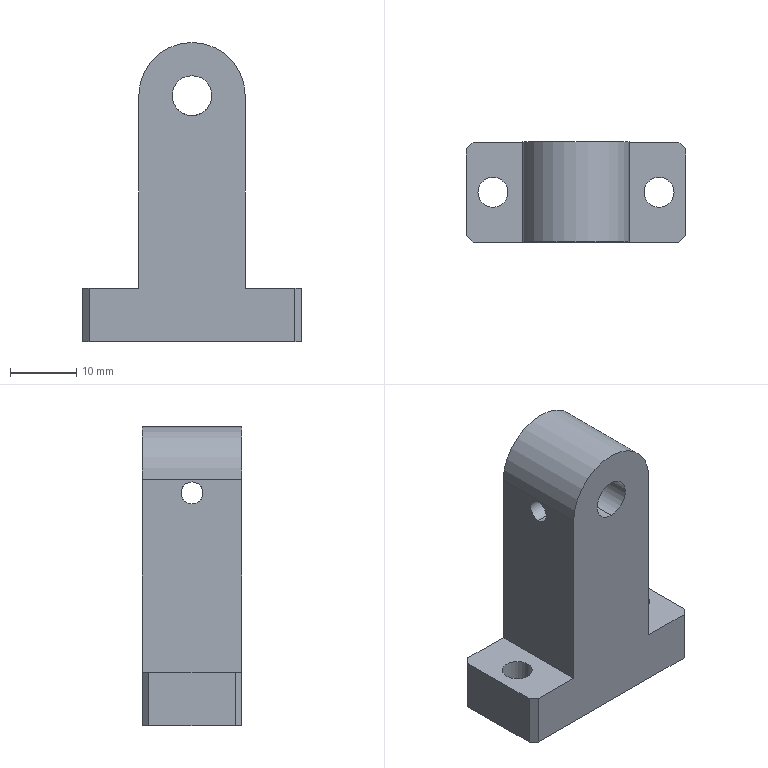Part | SolidWorks | features Chamfer 1, Extrusion 1, HoleWzd 1, ICE 1 | 1 solid | 22 faces | box 33 x 15 x 45 mm | volume 11629 mm3 | plane 13 | cylinder 9 | commonest cylinder face diameters 4.5 x4 3.3 x2 6 x2 16 x1
STEP:
#1=CARTESIAN_POINT('',(10.25,0.,-37.));
#2=VERTEX_POINT('',#1);
#3=CARTESIAN_POINT('',(14.75,0.,-37.));
#4=VERTEX_POINT('',#3);
#5=CARTESIAN_POINT('',(12.5,0.,-37.));
#6=DIRECTION('',(0.,0.,1.));
#7=DIRECTION('',(1.,0.,0.));
#8=AXIS2_PLACEMENT_3D('',#5,#6,#7);
#9=CIRCLE('',#8,2.25);
#10=EDGE_CURVE('',#2,#4,#9,.T.);
#11=ORIENTED_EDGE('',*,*,#10,.F.);
#12=CARTESIAN_POINT('',(10.25,0.,-29.));
#13=VERTEX_POINT('',#12);
#14=CARTESIAN_POINT('',(10.25,0.,-39.));
#15=DIRECTION('',(0.,0.,1.));
#16=VECTOR('',#15,1000.);
#17=LINE('',#14,#16);
#18=EDGE_CURVE('',#2,#13,#17,.T.);
#19=ORIENTED_EDGE('',*,*,#18,.T.);
#20=CARTESIAN_POINT('',(14.75,0.,-29.));
#21=VERTEX_POINT('',#20);
#22=CARTESIAN_POINT('',(12.5,0.,-29.));
#23=DIRECTION('',(0.,0.,1.));
#24=DIRECTION('',(-1.,0.,0.));
#25=AXIS2_PLACEMENT_3D('',#22,#23,#24);
#26=CIRCLE('',#25,2.25);
#27=EDGE_CURVE('',#13,#21,#26,.T.);
#28=ORIENTED_EDGE('',*,*,#27,.T.);
#29=CARTESIAN_POINT('',(14.75,0.,-39.));
#30=DIRECTION('',(0.,0.,1.));
#31=VECTOR('',#30,1000.);
#32=LINE('',#29,#31);
#33=EDGE_CURVE('',#4,#21,#32,.T.);
#34=ORIENTED_EDGE('',*,*,#33,.F.);
#35=EDGE_LOOP('',(#11,#19,#28,#34));
#36=FACE_OUTER_BOUND('',#35,.T.);
#37=CARTESIAN_POINT('',(12.5,0.,-39.));
#38=DIRECTION('',(0.,0.,1.));
#39=DIRECTION('',(1.,0.,0.));
#40=AXIS2_PLACEMENT_3D('',#37,#38,#39);
#41=CYLINDRICAL_SURFACE('',#40,2.25);
#42=ADVANCED_FACE('',(#36),#41,.F.);
#43=CARTESIAN_POINT('',(-14.75,0.,-37.));
#44=VERTEX_POINT('',#43);
#45=CARTESIAN_POINT('',(-10.25,0.,-37.));
#46=VERTEX_POINT('',#45);
#47=CARTESIAN_POINT('',(-12.5,0.,-37.));
#48=DIRECTION('',(0.,0.,1.));
#49=DIRECTION('',(1.,0.,0.));
#50=AXIS2_PLACEMENT_3D('',#47,#48,#49);
#51=CIRCLE('',#50,2.25);
#52=EDGE_CURVE('',#44,#46,#51,.T.);
#53=ORIENTED_EDGE('',*,*,#52,.F.);
#54=CARTESIAN_POINT('',(-14.75,0.,-29.));
#55=VERTEX_POINT('',#54);
#56=CARTESIAN_POINT('',(-14.75,0.,-39.));
#57=DIRECTION('',(0.,0.,1.));
#58=VECTOR('',#57,1000.);
#59=LINE('',#56,#58);
#60=EDGE_CURVE('',#44,#55,#59,.T.);
#61=ORIENTED_EDGE('',*,*,#60,.T.);
#62=CARTESIAN_POINT('',(-10.25,0.,-29.));
#63=VERTEX_POINT('',#62);
#64=CARTESIAN_POINT('',(-12.5,0.,-29.));
#65=DIRECTION('',(0.,0.,1.));
#66=DIRECTION('',(1.,0.,0.));
#67=AXIS2_PLACEMENT_3D('',#64,#65,#66);
#68=CIRCLE('',#67,2.25);
#69=EDGE_CURVE('',#55,#63,#68,.T.);
#70=ORIENTED_EDGE('',*,*,#69,.T.);
#71=CARTESIAN_POINT('',(-10.25,0.,-39.));
#72=DIRECTION('',(0.,0.,1.));
#73=VECTOR('',#72,1000.);
#74=LINE('',#71,#73);
#75=EDGE_CURVE('',#46,#63,#74,.T.);
#76=ORIENTED_EDGE('',*,*,#75,.F.);
#77=EDGE_LOOP('',(#53,#61,#70,#76));
#78=FACE_OUTER_BOUND('',#77,.T.);
#79=CARTESIAN_POINT('',(-12.5,0.,-39.));
#80=DIRECTION('',(0.,0.,1.));
#81=DIRECTION('',(1.,0.,0.));
#82=AXIS2_PLACEMENT_3D('',#79,#80,#81);
#83=CYLINDRICAL_SURFACE('',#82,2.25);
#84=ADVANCED_FACE('',(#78),#83,.F.);
#85=CARTESIAN_POINT('',(-8.,0.,-0.35));
#86=VERTEX_POINT('',#85);
#87=CARTESIAN_POINT('',(-8.,0.,-3.65));
#88=VERTEX_POINT('',#87);
#89=CARTESIAN_POINT('',(-8.,0.,-2.));
#90=DIRECTION('',(1.,0.,0.));
#91=DIRECTION('',(0.,0.,-1.));
#92=AXIS2_PLACEMENT_3D('',#89,#90,#91);
#93=CIRCLE('',#92,1.65);
#94=EDGE_CURVE('',#86,#88,#93,.T.);
#95=ORIENTED_EDGE('',*,*,#94,.F.);
#96=CARTESIAN_POINT('',(-2.98,0.,-0.35));
#97=VERTEX_POINT('',#96);
#98=CARTESIAN_POINT('',(8.,0.,-0.35));
#99=DIRECTION('',(1.,0.,0.));
#100=VECTOR('',#99,1000.);
#101=LINE('',#98,#100);
#102=EDGE_CURVE('',#86,#97,#101,.T.);
#103=ORIENTED_EDGE('',*,*,#102,.T.);
#104=CARTESIAN_POINT('',(0.,-1.312,-3.));
#105=VERTEX_POINT('',#104);
#106=CARTESIAN_POINT('',(-2.98,0.,-0.35));
#107=CARTESIAN_POINT('',(-2.98,-0.1118,-0.35));
#108=CARTESIAN_POINT('',(-2.978,-0.2224,-0.3613));
#109=CARTESIAN_POINT('',(-2.973,-0.4388,-0.4056));
#110=CARTESIAN_POINT('',(-2.968,-0.5462,-0.4391));
#111=CARTESIAN_POINT('',(-2.954,-0.7501,-0.5262));
#112=CARTESIAN_POINT('',(-2.944,-0.8464,-0.5794));
#113=CARTESIAN_POINT('',(-2.917,-1.028,-0.7044));
#114=CARTESIAN_POINT('',(-2.899,-1.112,-0.7767));
#115=CARTESIAN_POINT('',(-2.83,-1.337,-1.01));
#116=CARTESIAN_POINT('',(-2.76,-1.453,-1.194));
#117=CARTESIAN_POINT('',(-2.617,-1.566,-1.471));
#118=CARTESIAN_POINT('',(-2.561,-1.595,-1.566));
#119=CARTESIAN_POINT('',(-2.441,-1.633,-1.748));
#120=CARTESIAN_POINT('',(-2.375,-1.644,-1.836));
#121=CARTESIAN_POINT('',(-2.161,-1.656,-2.093));
#122=CARTESIAN_POINT('',(-2.001,-1.637,-2.246));
#123=CARTESIAN_POINT('',(-1.653,-1.574,-2.513));
#124=CARTESIAN_POINT('',(-1.466,-1.53,-2.627));
#125=CARTESIAN_POINT('',(-1.075,-1.442,-2.809));
#126=CARTESIAN_POINT('',(-0.8686,-1.397,-2.88));
#127=CARTESIAN_POINT('',(-0.4403,-1.332,-2.976));
#128=CARTESIAN_POINT('',(-0.2224,-1.312,-3.));
#129=CARTESIAN_POINT('',(0.,-1.312,-3.));
#130=B_SPLINE_CURVE_WITH_KNOTS('',3,(#106,#107,#108,#109,#110,#111,#112,#113,#114,#115,#116,#117,#118,#119,#120,#121,#122,#123,#124,#125,#126,#127,#128,#129),.UNSPECIFIED.,.F.,.F.,(4,2,2,2,2,2,2,2,2,2,2,4),(0.005283,0.005614,0.005944,0.006274,0.006604,0.007264,0.007594,0.007924,0.008585,0.009245,0.009905,0.01057),.UNSPECIFIED.);
#131=EDGE_CURVE('',#97,#105,#130,.T.);
#132=ORIENTED_EDGE('',*,*,#131,.T.);
#133=CARTESIAN_POINT('',(2.98,0.,-0.35));
#134=VERTEX_POINT('',#133);
#135=CARTESIAN_POINT('',(0.,-1.312,-3.));
#136=CARTESIAN_POINT('',(0.2222,-1.312,-3.));
#137=CARTESIAN_POINT('',(0.4425,-1.332,-2.975));
#138=CARTESIAN_POINT('',(0.8684,-1.397,-2.88));
#139=CARTESIAN_POINT('',(1.077,-1.442,-2.808));
#140=CARTESIAN_POINT('',(1.664,-1.575,-2.533));
#141=CARTESIAN_POINT('',(2.021,-1.665,-2.261));
#142=CARTESIAN_POINT('',(2.377,-1.644,-1.834));
#143=CARTESIAN_POINT('',(2.442,-1.633,-1.746));
#144=CARTESIAN_POINT('',(2.562,-1.594,-1.564));
#145=CARTESIAN_POINT('',(2.617,-1.566,-1.47));
#146=CARTESIAN_POINT('',(2.713,-1.49,-1.285));
#147=CARTESIAN_POINT('',(2.754,-1.444,-1.194));
#148=CARTESIAN_POINT('',(2.824,-1.33,-1.018));
#149=CARTESIAN_POINT('',(2.853,-1.262,-0.9321));
#150=CARTESIAN_POINT('',(2.922,-1.037,-0.6987));
#151=CARTESIAN_POINT('',(2.947,-0.8511,-0.5693));
#152=CARTESIAN_POINT('',(2.968,-0.5462,-0.4391));
#153=CARTESIAN_POINT('',(2.973,-0.4385,-0.4055));
#154=CARTESIAN_POINT('',(2.978,-0.2214,-0.3612));
#155=CARTESIAN_POINT('',(2.98,-0.1114,-0.35));
#156=CARTESIAN_POINT('',(2.98,0.,-0.35));
#157=B_SPLINE_CURVE_WITH_KNOTS('',3,(#135,#136,#137,#138,#139,#140,#141,#142,#143,#144,#145,#146,#147,#148,#149,#150,#151,#152,#153,#154,#155,#156),.UNSPECIFIED.,.F.,.F.,(4,2,2,2,2,2,2,2,2,2,4),(0.01057,0.01123,0.01189,0.0132,0.01353,0.01386,0.01419,0.01452,0.01518,0.01551,0.01584),.UNSPECIFIED.);
#158=EDGE_CURVE('',#105,#134,#157,.T.);
#159=ORIENTED_EDGE('',*,*,#158,.T.);
#160=CARTESIAN_POINT('',(8.,0.,-0.35));
#161=VERTEX_POINT('',#160);
#162=CARTESIAN_POINT('',(8.,0.,-0.35));
#163=DIRECTION('',(1.,0.,0.));
#164=VECTOR('',#163,1000.);
#165=LINE('',#162,#164);
#166=EDGE_CURVE('',#134,#161,#165,.T.);
#167=ORIENTED_EDGE('',*,*,#166,.T.);
#168=CARTESIAN_POINT('',(8.,0.,-3.65));
#169=VERTEX_POINT('',#168);
#170=CARTESIAN_POINT('',(8.,0.,-2.));
#171=DIRECTION('',(1.,0.,0.));
#172=DIRECTION('',(0.,0.,-1.));
#173=AXIS2_PLACEMENT_3D('',#170,#171,#172);
#174=CIRCLE('',#173,1.65);
#175=EDGE_CURVE('',#161,#169,#174,.T.);
#176=ORIENTED_EDGE('',*,*,#175,.T.);
#177=CARTESIAN_POINT('',(8.,0.,-3.65));
#178=DIRECTION('',(1.,0.,0.));
#179=VECTOR('',#178,1000.);
#180=LINE('',#177,#179);
#181=EDGE_CURVE('',#88,#169,#180,.T.);
#182=ORIENTED_EDGE('',*,*,#181,.F.);
#183=EDGE_LOOP('',(#95,#103,#132,#159,#167,#176,#182));
#184=FACE_OUTER_BOUND('',#183,.T.);
#185=CARTESIAN_POINT('',(8.,0.,-2.));
#186=DIRECTION('',(1.,0.,0.));
#187=DIRECTION('',(0.,0.,-1.));
#188=AXIS2_PLACEMENT_3D('',#185,#186,#187);
#189=CYLINDRICAL_SURFACE('',#188,1.65);
#190=ADVANCED_FACE('',(#184),#189,.F.);
#191=CARTESIAN_POINT('',(0.,7.5,-3.));
#192=VERTEX_POINT('',#191);
#193=CARTESIAN_POINT('',(0.,7.5,3.));
#194=VERTEX_POINT('',#193);
#195=CARTESIAN_POINT('',(0.,7.5,0.));
#196=DIRECTION('',(0.,1.,0.));
#197=DIRECTION('',(0.,0.,1.));
#198=AXIS2_PLACEMENT_3D('',#195,#196,#197);
#199=CIRCLE('',#198,3.);
#200=EDGE_CURVE('',#192,#194,#199,.T.);
#201=ORIENTED_EDGE('',*,*,#200,.T.);
#202=CARTESIAN_POINT('',(0.,-7.5,3.));
#203=VERTEX_POINT('',#202);
#204=CARTESIAN_POINT('',(0.,7.5,3.));
#205=DIRECTION('',(0.,-1.,0.));
#206=VECTOR('',#205,1000.);
#207=LINE('',#204,#206);
#208=EDGE_CURVE('',#194,#203,#207,.T.);
#209=ORIENTED_EDGE('',*,*,#208,.T.);
#210=CARTESIAN_POINT('',(0.,-7.5,-3.));
#211=VERTEX_POINT('',#210);
#212=CARTESIAN_POINT('',(0.,-7.5,0.));
#213=DIRECTION('',(0.,1.,0.));
#214=DIRECTION('',(0.,0.,1.));
#215=AXIS2_PLACEMENT_3D('',#212,#213,#214);
#216=CIRCLE('',#215,3.);
#217=EDGE_CURVE('',#211,#203,#216,.T.);
#218=ORIENTED_EDGE('',*,*,#217,.F.);
#219=CARTESIAN_POINT('',(0.,7.5,-3.));
#220=DIRECTION('',(0.,-1.,0.));
#221=VECTOR('',#220,1000.);
#222=LINE('',#219,#221);
#223=EDGE_CURVE('',#105,#211,#222,.T.);
#224=ORIENTED_EDGE('',*,*,#223,.F.);
#225=ORIENTED_EDGE('',*,*,#131,.F.);
#226=CARTESIAN_POINT('',(0.,1.312,-3.));
#227=VERTEX_POINT('',#226);
#228=CARTESIAN_POINT('',(0.,1.312,-3.));
#229=CARTESIAN_POINT('',(-0.2233,1.312,-3.));
#230=CARTESIAN_POINT('',(-0.4413,1.332,-2.975));
#231=CARTESIAN_POINT('',(-0.8683,1.397,-2.88));
#232=CARTESIAN_POINT('',(-1.076,1.442,-2.809));
#233=CARTESIAN_POINT('',(-1.468,1.53,-2.625));
#234=CARTESIAN_POINT('',(-1.656,1.575,-2.511));
#235=CARTESIAN_POINT('',(-1.916,1.622,-2.311));
#236=CARTESIAN_POINT('',(-1.999,1.634,-2.24));
#237=CARTESIAN_POINT('',(-2.158,1.649,-2.087));
#238=CARTESIAN_POINT('',(-2.234,1.652,-2.005));
#239=CARTESIAN_POINT('',(-2.376,1.644,-1.835));
#240=CARTESIAN_POINT('',(-2.442,1.633,-1.747));
#241=CARTESIAN_POINT('',(-2.562,1.594,-1.565));
#242=CARTESIAN_POINT('',(-2.617,1.566,-1.47));
#243=CARTESIAN_POINT('',(-2.712,1.491,-1.286));
#244=CARTESIAN_POINT('',(-2.753,1.444,-1.195));
#245=CARTESIAN_POINT('',(-2.824,1.33,-1.018));
#246=CARTESIAN_POINT('',(-2.853,1.263,-0.9325));
#247=CARTESIAN_POINT('',(-2.922,1.038,-0.6992));
#248=CARTESIAN_POINT('',(-2.947,0.8518,-0.5697));
#249=CARTESIAN_POINT('',(-2.968,0.5465,-0.4392));
#250=CARTESIAN_POINT('',(-2.973,0.4388,-0.4056));
#251=CARTESIAN_POINT('',(-2.978,0.222,-0.3613));
#252=CARTESIAN_POINT('',(-2.98,0.1118,-0.35));
#253=CARTESIAN_POINT('',(-2.98,0.,-0.35));
#254=B_SPLINE_CURVE_WITH_KNOTS('',3,(#228,#229,#230,#231,#232,#233,#234,#235,#236,#237,#238,#239,#240,#241,#242,#243,#244,#245,#246,#247,#248,#249,#250,#251,#252,#253),.UNSPECIFIED.,.F.,.F.,(4,2,2,2,2,2,2,2,2,2,2,2,4),(0.,0.0006604,0.001321,0.001981,0.002312,0.002642,0.002972,0.003302,0.003632,0.003963,0.004623,0.004953,0.005283),.UNSPECIFIED.);
#255=EDGE_CURVE('',#227,#97,#254,.T.);
#256=ORIENTED_EDGE('',*,*,#255,.F.);
#257=CARTESIAN_POINT('',(0.,7.5,-3.));
#258=DIRECTION('',(0.,-1.,0.));
#259=VECTOR('',#258,1000.);
#260=LINE('',#257,#259);
#261=EDGE_CURVE('',#192,#227,#260,.T.);
#262=ORIENTED_EDGE('',*,*,#261,.F.);
#263=EDGE_LOOP('',(#201,#209,#218,#224,#225,#256,#262));
#264=FACE_OUTER_BOUND('',#263,.T.);
#265=CARTESIAN_POINT('',(0.,7.5,0.));
#266=DIRECTION('',(0.,-1.,0.));
#267=DIRECTION('',(0.,0.,-1.));
#268=AXIS2_PLACEMENT_3D('',#265,#266,#267);
#269=CYLINDRICAL_SURFACE('',#268,3.);
#270=ADVANCED_FACE('',(#264),#269,.F.);
#271=CARTESIAN_POINT('',(15.5,7.5,-37.));
#272=VERTEX_POINT('',#271);
#273=CARTESIAN_POINT('',(-15.5,7.5,-37.));
#274=VERTEX_POINT('',#273);
#275=CARTESIAN_POINT('',(16.5,7.5,-37.));
#276=DIRECTION('',(-1.,0.,0.));
#277=VECTOR('',#276,1000.);
#278=LINE('',#275,#277);
#279=EDGE_CURVE('',#272,#274,#278,.T.);
#280=ORIENTED_EDGE('',*,*,#279,.T.);
#281=CARTESIAN_POINT('',(-15.5,7.5,-29.));
#282=VERTEX_POINT('',#281);
#283=CARTESIAN_POINT('',(-15.5,7.5,-29.));
#284=DIRECTION('',(0.,0.,1.));
#285=VECTOR('',#284,1000.);
#286=LINE('',#283,#285);
#287=EDGE_CURVE('',#274,#282,#286,.T.);
#288=ORIENTED_EDGE('',*,*,#287,.T.);
#289=CARTESIAN_POINT('',(-8.,7.5,-29.));
#290=VERTEX_POINT('',#289);
#291=CARTESIAN_POINT('',(-8.,7.5,-29.));
#292=DIRECTION('',(1.,0.,0.));
#293=VECTOR('',#292,1000.);
#294=LINE('',#291,#293);
#295=EDGE_CURVE('',#282,#290,#294,.T.);
#296=ORIENTED_EDGE('',*,*,#295,.T.);
#297=CARTESIAN_POINT('',(-8.,7.5,0.));
#298=VERTEX_POINT('',#297);
#299=CARTESIAN_POINT('',(-8.,7.5,0.));
#300=DIRECTION('',(0.,0.,1.));
#301=VECTOR('',#300,1000.);
#302=LINE('',#299,#301);
#303=EDGE_CURVE('',#290,#298,#302,.T.);
#304=ORIENTED_EDGE('',*,*,#303,.T.);
#305=CARTESIAN_POINT('',(8.,7.5,0.));
#306=VERTEX_POINT('',#305);
#307=CARTESIAN_POINT('',(0.,7.5,0.));
#308=DIRECTION('',(0.,1.,0.));
#309=DIRECTION('',(0.,0.,1.));
#310=AXIS2_PLACEMENT_3D('',#307,#308,#309);
#311=CIRCLE('',#310,8.);
#312=EDGE_CURVE('',#298,#306,#311,.T.);
#313=ORIENTED_EDGE('',*,*,#312,.T.);
#314=CARTESIAN_POINT('',(8.,7.5,-29.));
#315=VERTEX_POINT('',#314);
#316=CARTESIAN_POINT('',(8.,7.5,0.));
#317=DIRECTION('',(0.,0.,-1.));
#318=VECTOR('',#317,1000.);
#319=LINE('',#316,#318);
#320=EDGE_CURVE('',#306,#315,#319,.T.);
#321=ORIENTED_EDGE('',*,*,#320,.T.);
#322=CARTESIAN_POINT('',(15.5,7.5,-29.));
#323=VERTEX_POINT('',#322);
#324=CARTESIAN_POINT('',(8.,7.5,-29.));
#325=DIRECTION('',(1.,0.,0.));
#326=VECTOR('',#325,1000.);
#327=LINE('',#324,#326);
#328=EDGE_CURVE('',#315,#323,#327,.T.);
#329=ORIENTED_EDGE('',*,*,#328,.T.);
#330=CARTESIAN_POINT('',(15.5,7.5,-37.));
#331=DIRECTION('',(0.,0.,-1.));
#332=VECTOR('',#331,1000.);
#333=LINE('',#330,#332);
#334=EDGE_CURVE('',#323,#272,#333,.T.);
#335=ORIENTED_EDGE('',*,*,#334,.T.);
#336=EDGE_LOOP('',(#280,#288,#296,#304,#313,#321,#329,#335));
#337=FACE_OUTER_BOUND('',#336,.T.);
#338=ORIENTED_EDGE('',*,*,#200,.F.);
#339=CARTESIAN_POINT('',(0.,7.5,0.));
#340=DIRECTION('',(0.,1.,0.));
#341=DIRECTION('',(0.,0.,1.));
#342=AXIS2_PLACEMENT_3D('',#339,#340,#341);
#343=CIRCLE('',#342,3.);
#344=EDGE_CURVE('',#194,#192,#343,.T.);
#345=ORIENTED_EDGE('',*,*,#344,.F.);
#346=EDGE_LOOP('',(#338,#345));
#347=FACE_BOUND('',#346,.T.);
#348=CARTESIAN_POINT('',(0.,7.5,0.));
#349=DIRECTION('',(0.,1.,0.));
#350=DIRECTION('',(0.,0.,1.));
#351=AXIS2_PLACEMENT_3D('',#348,#349,#350);
#352=PLANE('',#351);
#353=ADVANCED_FACE('',(#337,#347),#352,.T.);
#354=CARTESIAN_POINT('',(-15.5,-7.5,-29.));
#355=VERTEX_POINT('',#354);
#356=CARTESIAN_POINT('',(-8.,-7.5,-29.));
#357=VERTEX_POINT('',#356);
#358=CARTESIAN_POINT('',(-8.,-7.5,-29.));
#359=DIRECTION('',(1.,0.,0.));
#360=VECTOR('',#359,1000.);
#361=LINE('',#358,#360);
#362=EDGE_CURVE('',#355,#357,#361,.T.);
#363=ORIENTED_EDGE('',*,*,#362,.F.);
#364=CARTESIAN_POINT('',(-15.5,-7.5,-37.));
#365=VERTEX_POINT('',#364);
#366=CARTESIAN_POINT('',(-15.5,-7.5,0.));
#367=DIRECTION('',(0.,0.,-1.));
#368=VECTOR('',#367,1000.);
#369=LINE('',#366,#368);
#370=EDGE_CURVE('',#355,#365,#369,.T.);
#371=ORIENTED_EDGE('',*,*,#370,.T.);
#372=CARTESIAN_POINT('',(15.5,-7.5,-37.));
#373=VERTEX_POINT('',#372);
#374=CARTESIAN_POINT('',(16.5,-7.5,-37.));
#375=DIRECTION('',(-1.,0.,0.));
#376=VECTOR('',#375,1000.);
#377=LINE('',#374,#376);
#378=EDGE_CURVE('',#373,#365,#377,.T.);
#379=ORIENTED_EDGE('',*,*,#378,.F.);
#380=CARTESIAN_POINT('',(15.5,-7.5,-29.));
#381=VERTEX_POINT('',#380);
#382=CARTESIAN_POINT('',(15.5,-7.5,0.));
#383=DIRECTION('',(0.,0.,1.));
#384=VECTOR('',#383,1000.);
#385=LINE('',#382,#384);
#386=EDGE_CURVE('',#373,#381,#385,.T.);
#387=ORIENTED_EDGE('',*,*,#386,.T.);
#388=CARTESIAN_POINT('',(8.,-7.5,-29.));
#389=VERTEX_POINT('',#388);
#390=CARTESIAN_POINT('',(8.,-7.5,-29.));
#391=DIRECTION('',(1.,0.,0.));
#392=VECTOR('',#391,1000.);
#393=LINE('',#390,#392);
#394=EDGE_CURVE('',#389,#381,#393,.T.);
#395=ORIENTED_EDGE('',*,*,#394,.F.);
#396=CARTESIAN_POINT('',(8.,-7.5,0.));
#397=VERTEX_POINT('',#396);
#398=CARTESIAN_POINT('',(8.,-7.5,0.));
#399=DIRECTION('',(0.,0.,-1.));
#400=VECTOR('',#399,1000.);
#401=LINE('',#398,#400);
#402=EDGE_CURVE('',#397,#389,#401,.T.);
#403=ORIENTED_EDGE('',*,*,#402,.F.);
#404=CARTESIAN_POINT('',(-8.,-7.5,0.));
#405=VERTEX_POINT('',#404);
#406=CARTESIAN_POINT('',(0.,-7.5,0.));
#407=DIRECTION('',(0.,1.,0.));
#408=DIRECTION('',(0.,0.,1.));
#409=AXIS2_PLACEMENT_3D('',#406,#407,#408);
#410=CIRCLE('',#409,8.);
#411=EDGE_CURVE('',#405,#397,#410,.T.);
#412=ORIENTED_EDGE('',*,*,#411,.F.);
#413=CARTESIAN_POINT('',(-8.,-7.5,0.));
#414=DIRECTION('',(0.,0.,1.));
#415=VECTOR('',#414,1000.);
#416=LINE('',#413,#415);
#417=EDGE_CURVE('',#357,#405,#416,.T.);
#418=ORIENTED_EDGE('',*,*,#417,.F.);
#419=EDGE_LOOP('',(#363,#371,#379,#387,#395,#403,#412,#418));
#420=FACE_OUTER_BOUND('',#419,.T.);
#421=ORIENTED_EDGE('',*,*,#217,.T.);
#422=CARTESIAN_POINT('',(0.,-7.5,0.));
#423=DIRECTION('',(0.,1.,0.));
#424=DIRECTION('',(0.,0.,1.));
#425=AXIS2_PLACEMENT_3D('',#422,#423,#424);
#426=CIRCLE('',#425,3.);
#427=EDGE_CURVE('',#203,#211,#426,.T.);
#428=ORIENTED_EDGE('',*,*,#427,.T.);
#429=EDGE_LOOP('',(#421,#428));
#430=FACE_BOUND('',#429,.T.);
#431=CARTESIAN_POINT('',(0.,-7.5,0.));
#432=DIRECTION('',(0.,1.,0.));
#433=DIRECTION('',(0.,0.,1.));
#434=AXIS2_PLACEMENT_3D('',#431,#432,#433);
#435=PLANE('',#434);
#436=ADVANCED_FACE('',(#420,#430),#435,.F.);
#437=ORIENTED_EDGE('',*,*,#411,.T.);
#438=CARTESIAN_POINT('',(8.,7.5,0.));
#439=DIRECTION('',(0.,-1.,0.));
#440=VECTOR('',#439,1000.);
#441=LINE('',#438,#440);
#442=EDGE_CURVE('',#306,#397,#441,.T.);
#443=ORIENTED_EDGE('',*,*,#442,.F.);
#444=ORIENTED_EDGE('',*,*,#312,.F.);
#445=CARTESIAN_POINT('',(-8.,7.5,0.));
#446=DIRECTION('',(0.,-1.,0.));
#447=VECTOR('',#446,1000.);
#448=LINE('',#445,#447);
#449=EDGE_CURVE('',#298,#405,#448,.T.);
#450=ORIENTED_EDGE('',*,*,#449,.T.);
#451=EDGE_LOOP('',(#437,#443,#444,#450));
#452=FACE_OUTER_BOUND('',#451,.T.);
#453=CARTESIAN_POINT('',(0.,7.5,0.));
#454=DIRECTION('',(0.,-1.,0.));
#455=DIRECTION('',(0.,0.,-1.));
#456=AXIS2_PLACEMENT_3D('',#453,#454,#455);
#457=CYLINDRICAL_SURFACE('',#456,8.);
#458=ADVANCED_FACE('',(#452),#457,.T.);
#459=CARTESIAN_POINT('',(8.,0.,-2.));
#460=DIRECTION('',(1.,0.,0.));
#461=DIRECTION('',(0.,0.,-1.));
#462=AXIS2_PLACEMENT_3D('',#459,#460,#461);
#463=CIRCLE('',#462,1.65);
#464=EDGE_CURVE('',#169,#161,#463,.T.);
#465=ORIENTED_EDGE('',*,*,#464,.F.);
#466=ORIENTED_EDGE('',*,*,#175,.F.);
#467=EDGE_LOOP('',(#465,#466));
#468=FACE_BOUND('',#467,.T.);
#469=ORIENTED_EDGE('',*,*,#402,.T.);
#470=CARTESIAN_POINT('',(8.,7.5,-29.));
#471=DIRECTION('',(0.,-1.,0.));
#472=VECTOR('',#471,1000.);
#473=LINE('',#470,#472);
#474=EDGE_CURVE('',#315,#389,#473,.T.);
#475=ORIENTED_EDGE('',*,*,#474,.F.);
#476=ORIENTED_EDGE('',*,*,#320,.F.);
#477=ORIENTED_EDGE('',*,*,#442,.T.);
#478=EDGE_LOOP('',(#469,#475,#476,#477));
#479=FACE_OUTER_BOUND('',#478,.T.);
#480=CARTESIAN_POINT('',(8.,7.5,0.));
#481=DIRECTION('',(-1.,0.,0.));
#482=DIRECTION('',(0.,0.,1.));
#483=AXIS2_PLACEMENT_3D('',#480,#481,#482);
#484=PLANE('',#483);
#485=ADVANCED_FACE('',(#468,#479),#484,.F.);
#486=CARTESIAN_POINT('',(12.5,0.,-29.));
#487=DIRECTION('',(0.,0.,1.));
#488=DIRECTION('',(-1.,0.,0.));
#489=AXIS2_PLACEMENT_3D('',#486,#487,#488);
#490=CIRCLE('',#489,2.25);
#491=EDGE_CURVE('',#21,#13,#490,.T.);
#492=ORIENTED_EDGE('',*,*,#491,.F.);
#493=ORIENTED_EDGE('',*,*,#27,.F.);
#494=EDGE_LOOP('',(#492,#493));
#495=FACE_BOUND('',#494,.T.);
#496=ORIENTED_EDGE('',*,*,#394,.T.);
#497=CARTESIAN_POINT('',(16.5,-6.5,-29.));
#498=VERTEX_POINT('',#497);
#499=CARTESIAN_POINT('',(16.5,-6.5,-29.));
#500=DIRECTION('',(0.7071,0.7071,0.));
#501=VECTOR('',#500,1000.);
#502=LINE('',#499,#501);
#503=EDGE_CURVE('',#381,#498,#502,.T.);
#504=ORIENTED_EDGE('',*,*,#503,.T.);
#505=CARTESIAN_POINT('',(16.5,6.5,-29.));
#506=VERTEX_POINT('',#505);
#507=CARTESIAN_POINT('',(16.5,7.5,-29.));
#508=DIRECTION('',(0.,-1.,0.));
#509=VECTOR('',#508,1000.);
#510=LINE('',#507,#509);
#511=EDGE_CURVE('',#506,#498,#510,.T.);
#512=ORIENTED_EDGE('',*,*,#511,.F.);
#513=CARTESIAN_POINT('',(15.5,7.5,-29.));
#514=DIRECTION('',(-0.7071,0.7071,0.));
#515=VECTOR('',#514,1000.);
#516=LINE('',#513,#515);
#517=EDGE_CURVE('',#506,#323,#516,.T.);
#518=ORIENTED_EDGE('',*,*,#517,.T.);
#519=ORIENTED_EDGE('',*,*,#328,.F.);
#520=ORIENTED_EDGE('',*,*,#474,.T.);
#521=EDGE_LOOP('',(#496,#504,#512,#518,#519,#520));
#522=FACE_OUTER_BOUND('',#521,.T.);
#523=CARTESIAN_POINT('',(8.,7.5,-29.));
#524=DIRECTION('',(0.,0.,-1.));
#525=DIRECTION('',(-1.,0.,0.));
#526=AXIS2_PLACEMENT_3D('',#523,#524,#525);
#527=PLANE('',#526);
#528=ADVANCED_FACE('',(#495,#522),#527,.F.);
#529=ORIENTED_EDGE('',*,*,#511,.T.);
#530=CARTESIAN_POINT('',(16.5,-6.5,-37.));
#531=VERTEX_POINT('',#530);
#532=CARTESIAN_POINT('',(16.5,-6.5,-29.));
#533=DIRECTION('',(0.,0.,-1.));
#534=VECTOR('',#533,1000.);
#535=LINE('',#532,#534);
#536=EDGE_CURVE('',#498,#531,#535,.T.);
#537=ORIENTED_EDGE('',*,*,#536,.T.);
#538=CARTESIAN_POINT('',(16.5,6.5,-37.));
#539=VERTEX_POINT('',#538);
#540=CARTESIAN_POINT('',(16.5,7.5,-37.));
#541=DIRECTION('',(0.,-1.,0.));
#542=VECTOR('',#541,1000.);
#543=LINE('',#540,#542);
#544=EDGE_CURVE('',#539,#531,#543,.T.);
#545=ORIENTED_EDGE('',*,*,#544,.F.);
#546=CARTESIAN_POINT('',(16.5,6.5,-29.));
#547=DIRECTION('',(0.,0.,1.));
#548=VECTOR('',#547,1000.);
#549=LINE('',#546,#548);
#550=EDGE_CURVE('',#539,#506,#549,.T.);
#551=ORIENTED_EDGE('',*,*,#550,.T.);
#552=EDGE_LOOP('',(#529,#537,#545,#551));
#553=FACE_OUTER_BOUND('',#552,.T.);
#554=CARTESIAN_POINT('',(16.5,7.5,-29.));
#555=DIRECTION('',(-1.,0.,0.));
#556=DIRECTION('',(0.,0.,1.));
#557=AXIS2_PLACEMENT_3D('',#554,#555,#556);
#558=PLANE('',#557);
#559=ADVANCED_FACE('',(#553),#558,.F.);
#560=CARTESIAN_POINT('',(12.5,0.,-37.));
#561=DIRECTION('',(0.,0.,1.));
#562=DIRECTION('',(1.,0.,0.));
#563=AXIS2_PLACEMENT_3D('',#560,#561,#562);
#564=CIRCLE('',#563,2.25);
#565=EDGE_CURVE('',#4,#2,#564,.T.);
#566=ORIENTED_EDGE('',*,*,#565,.T.);
#567=ORIENTED_EDGE('',*,*,#10,.T.);
#568=EDGE_LOOP('',(#566,#567));
#569=FACE_BOUND('',#568,.T.);
#570=CARTESIAN_POINT('',(-12.5,0.,-37.));
#571=DIRECTION('',(0.,0.,1.));
#572=DIRECTION('',(1.,0.,0.));
#573=AXIS2_PLACEMENT_3D('',#570,#571,#572);
#574=CIRCLE('',#573,2.25);
#575=EDGE_CURVE('',#46,#44,#574,.T.);
#576=ORIENTED_EDGE('',*,*,#575,.T.);
#577=ORIENTED_EDGE('',*,*,#52,.T.);
#578=EDGE_LOOP('',(#576,#577));
#579=FACE_BOUND('',#578,.T.);
#580=CARTESIAN_POINT('',(-16.5,6.5,-37.));
#581=VERTEX_POINT('',#580);
#582=CARTESIAN_POINT('',(-16.5,-6.5,-37.));
#583=VERTEX_POINT('',#582);
#584=CARTESIAN_POINT('',(-16.5,7.5,-37.));
#585=DIRECTION('',(0.,-1.,0.));
#586=VECTOR('',#585,1000.);
#587=LINE('',#584,#586);
#588=EDGE_CURVE('',#581,#583,#587,.T.);
#589=ORIENTED_EDGE('',*,*,#588,.F.);
#590=CARTESIAN_POINT('',(-15.5,7.5,-37.));
#591=DIRECTION('',(0.7071,0.7071,0.));
#592=VECTOR('',#591,1000.);
#593=LINE('',#590,#592);
#594=EDGE_CURVE('',#581,#274,#593,.T.);
#595=ORIENTED_EDGE('',*,*,#594,.T.);
#596=ORIENTED_EDGE('',*,*,#279,.F.);
#597=CARTESIAN_POINT('',(15.5,7.5,-37.));
#598=DIRECTION('',(0.7071,-0.7071,0.));
#599=VECTOR('',#598,1000.);
#600=LINE('',#597,#599);
#601=EDGE_CURVE('',#272,#539,#600,.T.);
#602=ORIENTED_EDGE('',*,*,#601,.T.);
#603=ORIENTED_EDGE('',*,*,#544,.T.);
#604=CARTESIAN_POINT('',(16.5,-6.5,-37.));
#605=DIRECTION('',(-0.7071,-0.7071,0.));
#606=VECTOR('',#605,1000.);
#607=LINE('',#604,#606);
#608=EDGE_CURVE('',#531,#373,#607,.T.);
#609=ORIENTED_EDGE('',*,*,#608,.T.);
#610=ORIENTED_EDGE('',*,*,#378,.T.);
#611=CARTESIAN_POINT('',(-16.5,-6.5,-37.));
#612=DIRECTION('',(-0.7071,0.7071,0.));
#613=VECTOR('',#612,1000.);
#614=LINE('',#611,#613);
#615=EDGE_CURVE('',#365,#583,#614,.T.);
#616=ORIENTED_EDGE('',*,*,#615,.T.);
#617=EDGE_LOOP('',(#589,#595,#596,#602,#603,#609,#610,#616));
#618=FACE_OUTER_BOUND('',#617,.T.);
#619=CARTESIAN_POINT('',(16.5,7.5,-37.));
#620=DIRECTION('',(0.,0.,1.));
#621=DIRECTION('',(1.,0.,0.));
#622=AXIS2_PLACEMENT_3D('',#619,#620,#621);
#623=PLANE('',#622);
#624=ADVANCED_FACE('',(#569,#579,#618),#623,.F.);
#625=CARTESIAN_POINT('',(-16.5,6.5,-29.));
#626=VERTEX_POINT('',#625);
#627=CARTESIAN_POINT('',(-16.5,-6.5,-29.));
#628=VERTEX_POINT('',#627);
#629=CARTESIAN_POINT('',(-16.5,7.5,-29.));
#630=DIRECTION('',(0.,-1.,0.));
#631=VECTOR('',#630,1000.);
#632=LINE('',#629,#631);
#633=EDGE_CURVE('',#626,#628,#632,.T.);
#634=ORIENTED_EDGE('',*,*,#633,.F.);
#635=CARTESIAN_POINT('',(-16.5,6.5,-37.));
#636=DIRECTION('',(0.,0.,-1.));
#637=VECTOR('',#636,1000.);
#638=LINE('',#635,#637);
#639=EDGE_CURVE('',#626,#581,#638,.T.);
#640=ORIENTED_EDGE('',*,*,#639,.T.);
#641=ORIENTED_EDGE('',*,*,#588,.T.);
#642=CARTESIAN_POINT('',(-16.5,-6.5,-29.));
#643=DIRECTION('',(0.,0.,1.));
#644=VECTOR('',#643,1000.);
#645=LINE('',#642,#644);
#646=EDGE_CURVE('',#583,#628,#645,.T.);
#647=ORIENTED_EDGE('',*,*,#646,.T.);
#648=EDGE_LOOP('',(#634,#640,#641,#647));
#649=FACE_OUTER_BOUND('',#648,.T.);
#650=CARTESIAN_POINT('',(-16.5,7.5,-29.));
#651=DIRECTION('',(1.,0.,0.));
#652=DIRECTION('',(0.,0.,-1.));
#653=AXIS2_PLACEMENT_3D('',#650,#651,#652);
#654=PLANE('',#653);
#655=ADVANCED_FACE('',(#649),#654,.F.);
#656=CARTESIAN_POINT('',(-12.5,0.,-29.));
#657=DIRECTION('',(0.,0.,1.));
#658=DIRECTION('',(1.,0.,0.));
#659=AXIS2_PLACEMENT_3D('',#656,#657,#658);
#660=CIRCLE('',#659,2.25);
#661=EDGE_CURVE('',#63,#55,#660,.T.);
#662=ORIENTED_EDGE('',*,*,#661,.F.);
#663=ORIENTED_EDGE('',*,*,#69,.F.);
#664=EDGE_LOOP('',(#662,#663));
#665=FACE_BOUND('',#664,.T.);
#666=ORIENTED_EDGE('',*,*,#295,.F.);
#667=CARTESIAN_POINT('',(-15.5,7.5,-29.));
#668=DIRECTION('',(-0.7071,-0.7071,0.));
#669=VECTOR('',#668,1000.);
#670=LINE('',#667,#669);
#671=EDGE_CURVE('',#282,#626,#670,.T.);
#672=ORIENTED_EDGE('',*,*,#671,.T.);
#673=ORIENTED_EDGE('',*,*,#633,.T.);
#674=CARTESIAN_POINT('',(-16.5,-6.5,-29.));
#675=DIRECTION('',(0.7071,-0.7071,0.));
#676=VECTOR('',#675,1000.);
#677=LINE('',#674,#676);
#678=EDGE_CURVE('',#628,#355,#677,.T.);
#679=ORIENTED_EDGE('',*,*,#678,.T.);
#680=ORIENTED_EDGE('',*,*,#362,.T.);
#681=CARTESIAN_POINT('',(-8.,7.5,-29.));
#682=DIRECTION('',(0.,-1.,0.));
#683=VECTOR('',#682,1000.);
#684=LINE('',#681,#683);
#685=EDGE_CURVE('',#290,#357,#684,.T.);
#686=ORIENTED_EDGE('',*,*,#685,.F.);
#687=EDGE_LOOP('',(#666,#672,#673,#679,#680,#686));
#688=FACE_OUTER_BOUND('',#687,.T.);
#689=CARTESIAN_POINT('',(-8.,7.5,-29.));
#690=DIRECTION('',(0.,0.,-1.));
#691=DIRECTION('',(-1.,0.,0.));
#692=AXIS2_PLACEMENT_3D('',#689,#690,#691);
#693=PLANE('',#692);
#694=ADVANCED_FACE('',(#665,#688),#693,.F.);
#695=CARTESIAN_POINT('',(-8.,0.,-2.));
#696=DIRECTION('',(1.,0.,0.));
#697=DIRECTION('',(0.,0.,-1.));
#698=AXIS2_PLACEMENT_3D('',#695,#696,#697);
#699=CIRCLE('',#698,1.65);
#700=EDGE_CURVE('',#88,#86,#699,.T.);
#701=ORIENTED_EDGE('',*,*,#700,.T.);
#702=ORIENTED_EDGE('',*,*,#94,.T.);
#703=EDGE_LOOP('',(#701,#702));
#704=FACE_BOUND('',#703,.T.);
#705=ORIENTED_EDGE('',*,*,#417,.T.);
#706=ORIENTED_EDGE('',*,*,#449,.F.);
#707=ORIENTED_EDGE('',*,*,#303,.F.);
#708=ORIENTED_EDGE('',*,*,#685,.T.);
#709=EDGE_LOOP('',(#705,#706,#707,#708));
#710=FACE_OUTER_BOUND('',#709,.T.);
#711=CARTESIAN_POINT('',(-8.,7.5,0.));
#712=DIRECTION('',(1.,0.,0.));
#713=DIRECTION('',(0.,0.,-1.));
#714=AXIS2_PLACEMENT_3D('',#711,#712,#713);
#715=PLANE('',#714);
#716=ADVANCED_FACE('',(#704,#710),#715,.F.);
#717=ORIENTED_EDGE('',*,*,#208,.F.);
#718=ORIENTED_EDGE('',*,*,#344,.T.);
#719=ORIENTED_EDGE('',*,*,#261,.T.);
#720=CARTESIAN_POINT('',(2.98,0.,-0.35));
#721=CARTESIAN_POINT('',(2.98,0.2227,-0.35));
#722=CARTESIAN_POINT('',(2.975,0.4434,-0.3952));
#723=CARTESIAN_POINT('',(2.954,0.7502,-0.5262));
#724=CARTESIAN_POINT('',(2.944,0.8465,-0.5794));
#725=CARTESIAN_POINT('',(2.917,1.027,-0.704));
#726=CARTESIAN_POINT('',(2.899,1.112,-0.7764));
#727=CARTESIAN_POINT('',(2.83,1.337,-1.01));
#728=CARTESIAN_POINT('',(2.76,1.453,-1.193));
#729=CARTESIAN_POINT('',(2.617,1.566,-1.471));
#730=CARTESIAN_POINT('',(2.562,1.594,-1.565));
#731=CARTESIAN_POINT('',(2.441,1.633,-1.747));
#732=CARTESIAN_POINT('',(2.376,1.644,-1.836));
#733=CARTESIAN_POINT('',(2.02,1.664,-2.262));
#734=CARTESIAN_POINT('',(1.662,1.574,-2.535));
#735=CARTESIAN_POINT('',(1.077,1.442,-2.808));
#736=CARTESIAN_POINT('',(0.8716,1.398,-2.879));
#737=CARTESIAN_POINT('',(0.442,1.332,-2.975));
#738=CARTESIAN_POINT('',(0.223,1.312,-3.));
#739=CARTESIAN_POINT('',(0.,1.312,-3.));
#740=B_SPLINE_CURVE_WITH_KNOTS('',3,(#720,#721,#722,#723,#724,#725,#726,#727,#728,#729,#730,#731,#732,#733,#734,#735,#736,#737,#738,#739),.UNSPECIFIED.,.F.,.F.,(4,2,2,2,2,2,2,2,2,4),(0.01584,0.0165,0.01683,0.01716,0.01782,0.01815,0.01848,0.0198,0.02046,0.02112),.UNSPECIFIED.);
#741=EDGE_CURVE('',#134,#227,#740,.T.);
#742=ORIENTED_EDGE('',*,*,#741,.F.);
#743=ORIENTED_EDGE('',*,*,#158,.F.);
#744=ORIENTED_EDGE('',*,*,#223,.T.);
#745=ORIENTED_EDGE('',*,*,#427,.F.);
#746=EDGE_LOOP('',(#717,#718,#719,#742,#743,#744,#745));
#747=FACE_OUTER_BOUND('',#746,.T.);
#748=CARTESIAN_POINT('',(0.,7.5,0.));
#749=DIRECTION('',(0.,-1.,0.));
#750=DIRECTION('',(0.,0.,-1.));
#751=AXIS2_PLACEMENT_3D('',#748,#749,#750);
#752=CYLINDRICAL_SURFACE('',#751,3.);
#753=ADVANCED_FACE('',(#747),#752,.F.);
#754=ORIENTED_EDGE('',*,*,#102,.F.);
#755=ORIENTED_EDGE('',*,*,#700,.F.);
#756=ORIENTED_EDGE('',*,*,#181,.T.);
#757=ORIENTED_EDGE('',*,*,#464,.T.);
#758=ORIENTED_EDGE('',*,*,#166,.F.);
#759=ORIENTED_EDGE('',*,*,#741,.T.);
#760=ORIENTED_EDGE('',*,*,#255,.T.);
#761=EDGE_LOOP('',(#754,#755,#756,#757,#758,#759,#760));
#762=FACE_OUTER_BOUND('',#761,.T.);
#763=CARTESIAN_POINT('',(8.,0.,-2.));
#764=DIRECTION('',(1.,0.,0.));
#765=DIRECTION('',(0.,0.,-1.));
#766=AXIS2_PLACEMENT_3D('',#763,#764,#765);
#767=CYLINDRICAL_SURFACE('',#766,1.65);
#768=ADVANCED_FACE('',(#762),#767,.F.);
#769=ORIENTED_EDGE('',*,*,#60,.F.);
#770=ORIENTED_EDGE('',*,*,#575,.F.);
#771=ORIENTED_EDGE('',*,*,#75,.T.);
#772=ORIENTED_EDGE('',*,*,#661,.T.);
#773=EDGE_LOOP('',(#769,#770,#771,#772));
#774=FACE_OUTER_BOUND('',#773,.T.);
#775=CARTESIAN_POINT('',(-12.5,0.,-39.));
#776=DIRECTION('',(0.,0.,1.));
#777=DIRECTION('',(1.,0.,0.));
#778=AXIS2_PLACEMENT_3D('',#775,#776,#777);
#779=CYLINDRICAL_SURFACE('',#778,2.25);
#780=ADVANCED_FACE('',(#774),#779,.F.);
#781=ORIENTED_EDGE('',*,*,#18,.F.);
#782=ORIENTED_EDGE('',*,*,#565,.F.);
#783=ORIENTED_EDGE('',*,*,#33,.T.);
#784=ORIENTED_EDGE('',*,*,#491,.T.);
#785=EDGE_LOOP('',(#781,#782,#783,#784));
#786=FACE_OUTER_BOUND('',#785,.T.);
#787=CARTESIAN_POINT('',(12.5,0.,-39.));
#788=DIRECTION('',(0.,0.,1.));
#789=DIRECTION('',(1.,0.,0.));
#790=AXIS2_PLACEMENT_3D('',#787,#788,#789);
#791=CYLINDRICAL_SURFACE('',#790,2.25);
#792=ADVANCED_FACE('',(#786),#791,.F.);
#793=ORIENTED_EDGE('',*,*,#594,.F.);
#794=ORIENTED_EDGE('',*,*,#639,.F.);
#795=ORIENTED_EDGE('',*,*,#671,.F.);
#796=ORIENTED_EDGE('',*,*,#287,.F.);
#797=EDGE_LOOP('',(#793,#794,#795,#796));
#798=FACE_OUTER_BOUND('',#797,.T.);
#799=CARTESIAN_POINT('',(-15.5,7.5,0.));
#800=DIRECTION('',(-0.7071,0.7071,0.));
#801=DIRECTION('',(0.,0.,-1.));
#802=AXIS2_PLACEMENT_3D('',#799,#800,#801);
#803=PLANE('',#802);
#804=ADVANCED_FACE('',(#798),#803,.T.);
#805=ORIENTED_EDGE('',*,*,#615,.F.);
#806=ORIENTED_EDGE('',*,*,#370,.F.);
#807=ORIENTED_EDGE('',*,*,#678,.F.);
#808=ORIENTED_EDGE('',*,*,#646,.F.);
#809=EDGE_LOOP('',(#805,#806,#807,#808));
#810=FACE_OUTER_BOUND('',#809,.T.);
#811=CARTESIAN_POINT('',(-16.5,-6.5,-29.));
#812=DIRECTION('',(0.7071,0.7071,0.));
#813=DIRECTION('',(0.,0.,1.));
#814=AXIS2_PLACEMENT_3D('',#811,#812,#813);
#815=PLANE('',#814);
#816=ADVANCED_FACE('',(#810),#815,.F.);
#817=ORIENTED_EDGE('',*,*,#503,.F.);
#818=ORIENTED_EDGE('',*,*,#386,.F.);
#819=ORIENTED_EDGE('',*,*,#608,.F.);
#820=ORIENTED_EDGE('',*,*,#536,.F.);
#821=EDGE_LOOP('',(#817,#818,#819,#820));
#822=FACE_OUTER_BOUND('',#821,.T.);
#823=CARTESIAN_POINT('',(16.5,-6.5,-29.));
#824=DIRECTION('',(-0.7071,0.7071,0.));
#825=DIRECTION('',(0.,0.,-1.));
#826=AXIS2_PLACEMENT_3D('',#823,#824,#825);
#827=PLANE('',#826);
#828=ADVANCED_FACE('',(#822),#827,.F.);
#829=ORIENTED_EDGE('',*,*,#517,.F.);
#830=ORIENTED_EDGE('',*,*,#550,.F.);
#831=ORIENTED_EDGE('',*,*,#601,.F.);
#832=ORIENTED_EDGE('',*,*,#334,.F.);
#833=EDGE_LOOP('',(#829,#830,#831,#832));
#834=FACE_OUTER_BOUND('',#833,.T.);
#835=CARTESIAN_POINT('',(15.5,7.5,0.));
#836=DIRECTION('',(0.7071,0.7071,0.));
#837=DIRECTION('',(0.,0.,1.));
#838=AXIS2_PLACEMENT_3D('',#835,#836,#837);
#839=PLANE('',#838);
#840=ADVANCED_FACE('',(#834),#839,.T.);
#841=CLOSED_SHELL('',(#42,#84,#190,#270,#353,#436,#458,#485,#528,#559,#624,#655,#694,#716,#753,#768,#780,#792,#804,#816,#828,#840));
#842=MANIFOLD_SOLID_BREP('',#841);
#843=CARTESIAN_POINT('',(0.,0.,0.));
#844=DIRECTION('',(0.,0.,1.));
#845=DIRECTION('',(1.,0.,0.));
#846=AXIS2_PLACEMENT_3D('',#843,#844,#845);
#847=(LENGTH_UNIT()NAMED_UNIT(*)SI_UNIT(.MILLI.,.METRE.));
#848=UNCERTAINTY_MEASURE_WITH_UNIT(LENGTH_MEASURE(0.00001),#847,'','');
#849=(NAMED_UNIT(*)PLANE_ANGLE_UNIT()SI_UNIT($,.RADIAN.));
#850=(NAMED_UNIT(*)SI_UNIT($,.STERADIAN.)SOLID_ANGLE_UNIT());
#851=(GEOMETRIC_REPRESENTATION_CONTEXT(3)GLOBAL_UNCERTAINTY_ASSIGNED_CONTEXT((#848))GLOBAL_UNIT_ASSIGNED_CONTEXT((#847,#849,#850))REPRESENTATION_CONTEXT('',''));
#852=ADVANCED_BREP_SHAPE_REPRESENTATION('',(#842,#846),#851);